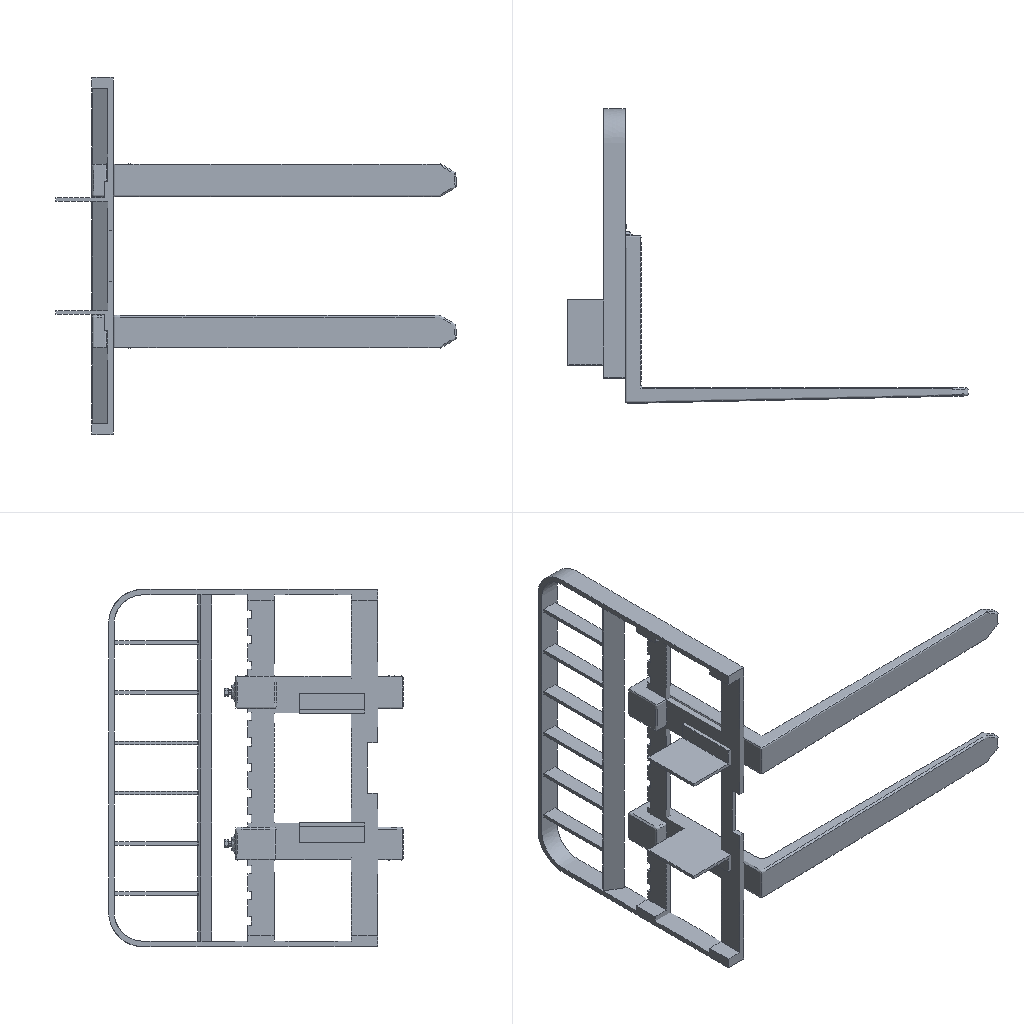Simulation study | ansys workbench
Set-up summary:
category,name,step,type,value,unit,region
solver,ansys_workbench
units,SI m-kg-s (Pa),,stated,"/units,MKS"
analysis,LS1,,static
load_step,LS1,LS1,static,nsubst=1; time=1
mesh,nodes,,,107409
mesh,elements,,,69133
element_type,SOLID187,,,59245
element_type,TARGE170,,,4743
element_type,CONTA174,,,4743
element_type,SOLID186,,,390
element_type,SURF154,,,12
material,Structural Steel,,E,2e+11,Pa
material,Structural Steel,,nu,0.3
material,Structural Steel,,density,7850,kg m^-3
material,Structural Steel,,conductivity,60.5,W m^-1 C^-1
material,Structural Steel,,specific_heat,434,J kg^-1 C^-1
material,Structural Steel,,cte,1.2e-05,C^-1
material,Structural Steel,,permeability,10000
material,Structural Steel,,resistivity,1.7e-07,kg m^3 A^-2 s^-3
load,Define Force Using Surface Effect Elements,LS1,surface-effect pres face 1,260906,,SURF154 #17
load,Define Force Using Surface Effect Elements,LS1,surface-effect pres face 2,-1.18334e+07,,SURF154 #17
bc,Fixed Supports,model,fixed,[dofs=ALL],,_FIXEDSU
contact,Contact Region 69,,bonded (always),element=CONTA174
contact,Contact Region 70,,bonded (always),element=CONTA174
contact,Contact Region 71,,bonded (always),element=CONTA174
contact,Contact Region 72,,bonded (always),element=CONTA174
contact,Contact Region 73,,bonded (always),element=CONTA174
named_set,_FIXEDSU,,node,1202
Ansys APDL input file, long lists of numbers shortened:
/batch
/config,noeldb,1     ! force off writing results to database
*get,_wallstrt,active,,time,wall
! ANSYS input file written by Workbench version 2024 R2
! File used for geometry attach:
/title,wbnew--____ (A5)
! ****** Begin Custom Load Command Snippet ******
/COM, ACT Extensions:
/COM,     LSDYNA, 2024.2
/COM,/COM,     ANSYSMotion, 2024.2
/COM,
! ****** End   Custom Load Command Snippet ******
*DIM,_wb_ProjectScratch_dir,string,248
_wb_ProjectScratch_dir(1) = ''
*DIM,_wb_SolverFiles_dir,string,248
_wb_SolverFiles_dir(1) = ''
*DIM,_wb_userfiles_dir,string,248
_wb_userfiles_dir(1) = ''
/com,--- Data in consistent MKS units. See Solving Units in the help system for more information.
/units,MKS
/nopr
/wb,file,start              !  signify a WB generated input file
/prep7
! Turn off shape checking because checks already performed inside WB mesher.
! See help system for more information.
SHPP,OFF,,NOWARN
/nolist
etcon,set             ! allow ANSYS to choose best KEYOP's for 180x elements, resets any applicable keyopt to MAPDL defaults
/com,*********** Nodes for the whole assembly ***********
nblock,3,,118149
(1i9,3e20.9e3)
   104394     6.272957041E-01     1.699172414E-01    -2.293882759E-01
! (107408 more lines like these left out)
-1
/wb,elem,start            !  set before creation of elements
/com,*********** Elements for Body 1 'EMPILHADEIRA_5T_ALTERADA_ASM_1_ASM|_______FORKLIFT_ASM_1_ASM|S_X_F3LIDO142_1|S_X_F3LIDO142_1' ***********
et,1,187
eblock,19,solid,,12218
(19i9)
        1        1        1        1        0        0        0        0       10        0        1      677     3666     4225     3693     8683    23642     8685     8684
! (24435 more lines like these left out)
-1
/com,*********** Elements for Body 2 'EMPILHADEIRA_5T_ALTERADA_ASM_1_ASM|_______FORKLIFT_ASM_1_ASM|S_X_F3LIDO143_1|S_X_F3LIDO143_1' ***********
et,2,187
eblock,19,solid,,18825
(19i9)
        2        2        2        2        0        0        0        0       10        0    12219    28224    29068    28415    28445    53792    54603    53786    53789
! (37649 more lines like these left out)
-1
/com,*********** Elements for Body 3 'EMPILHADEIRA_5T_ALTERADA_ASM_1_ASM|_______FORKLIFT_ASM_1_ASM|S_X_F3LIDO144_1|S_X_F3LIDO144_1' ***********
et,3,187
eblock,19,solid,,17962
(19i9)
        3        3        3        3        0        0        0        0       10        0    31044    58834    59006    59826    59181    82217    83239    82226    82221
! (35923 more lines like these left out)
-1
/com,*********** Elements for Body 4 'EMPILHADEIRA_5T_ALTERADA_ASM_1_ASM|_______FORKLIFT_ASM_1_ASM|S_X_F3LIDO152_1|S_X_F3LIDO152_1' ***********
et,4,187
eblock,19,solid,,10240
(19i9)
        4        4        4        4        0        0        0        0       10        0    49006    85338    88197    87604    88134    90879   103683    90876    90878
! (20479 more lines like these left out)
-1
/com,*********** Elements for Body 5 'EMPILHADEIRA_5T_ALTERADA_ASM_1_ASM|_______FORKLIFT_ASM_1_ASM|S_X_F3LIDO153_1|S_X_F3LIDO153_1' ***********
et,5,186
keyo,5,2,1          ! set full integration on SOLID186
eblock,19,solid,,195
(19i9)
        5        5        5        5        0        0        0        0       20        0    59246   104749   104790   104788   104775   104763   104838   104789   104776
! (389 more lines like these left out)
-1
/com,*********** Elements for Body 6 'EMPILHADEIRA_5T_ALTERADA_ASM_1_ASM|_______FORKLIFT_ASM_1_ASM|S_X_F3LIDO154_1|S_X_F3LIDO154_1' ***********
et,6,186
keyo,6,2,1          ! set full integration on SOLID186
eblock,19,solid,,195
(19i9)
        6        6        6        6        0        0        0        0       20        0    59441   106269   106311   106309   106296   106281   106349   106310   106297
! (389 more lines like these left out)
-1
/wb,elem,end               !  done creating elements
/com,*********** Send User Defined Coordinate System(s) ***********
csys,0
toffst,273.15,      ! Temperature offset from absolute zero
/com,*********** Set Reference Temperature ***********
tref,22.
/wb,mat,start              !  starting to send materials
/com,*********** Send Materials ***********
Temperature = 'TEMP' ! Temperature
MP,DENS,1,7850,	! kg m^-3
MP,ALPX,1,1.2e-05,	! C^-1
MP,C,1,434,	! J kg^-1 C^-1
MP,KXX,1,60.5,	! W m^-1 C^-1
MP,RSVX,1,1.7e-07,	! kg m^3 A^-2 s^-3
MP,EX,1,200000000000,	! Pa
MP,NUXY,1,0.3,
MP,MURX,1,10000,
Temperature = 'TEMP' ! Temperature
MP,DENS,2,7850,	! kg m^-3
MP,ALPX,2,1.2e-05,	! C^-1
MP,C,2,434,	! J kg^-1 C^-1
MP,KXX,2,60.5,	! W m^-1 C^-1
MP,RSVX,2,1.7e-07,	! kg m^3 A^-2 s^-3
MP,EX,2,200000000000,	! Pa
MP,NUXY,2,0.3,
MP,MURX,2,10000,
Temperature = 'TEMP' ! Temperature
MP,DENS,3,7850,	! kg m^-3
MP,ALPX,3,1.2e-05,	! C^-1
MP,C,3,434,	! J kg^-1 C^-1
MP,KXX,3,60.5,	! W m^-1 C^-1
MP,RSVX,3,1.7e-07,	! kg m^3 A^-2 s^-3
MP,EX,3,200000000000,	! Pa
MP,NUXY,3,0.3,
MP,MURX,3,10000,
Temperature = 'TEMP' ! Temperature
MP,DENS,4,7850,	! kg m^-3
MP,ALPX,4,1.2e-05,	! C^-1
MP,C,4,434,	! J kg^-1 C^-1
MP,KXX,4,60.5,	! W m^-1 C^-1
MP,RSVX,4,1.7e-07,	! kg m^3 A^-2 s^-3
MP,EX,4,200000000000,	! Pa
MP,NUXY,4,0.3,
MP,MURX,4,10000,
Temperature = 'TEMP' ! Temperature
MP,DENS,5,7850,	! kg m^-3
MP,ALPX,5,1.2e-05,	! C^-1
MP,C,5,434,	! J kg^-1 C^-1
MP,KXX,5,60.5,	! W m^-1 C^-1
MP,RSVX,5,1.7e-07,	! kg m^3 A^-2 s^-3
MP,EX,5,200000000000,	! Pa
MP,NUXY,5,0.3,
MP,MURX,5,10000,
Temperature = 'TEMP' ! Temperature
MP,DENS,6,7850,	! kg m^-3
MP,ALPX,6,1.2e-05,	! C^-1
MP,C,6,434,	! J kg^-1 C^-1
MP,KXX,6,60.5,	! W m^-1 C^-1
MP,RSVX,6,1.7e-07,	! kg m^3 A^-2 s^-3
MP,EX,6,200000000000,	! Pa
MP,NUXY,6,0.3,
MP,MURX,6,10000,
/wb,mat,end                !  done sending materials
!************************* Model Summary ********************
!EMPILHADEIRA_5T_ALTERADA_ASM_1_ASM|_______FORKLIFT_ASM_1_ASM|S_X_F3LIDO142_1|S_X_F3LIDO142_1,	ç»æé¢,	matid,	1
!EMPILHADEIRA_5T_ALTERADA_ASM_1_ASM|_______FORKLIFT_ASM_1_ASM|S_X_F3LIDO143_1|S_X_F3LIDO143_1,	ç»æé¢,	matid,	2
!EMPILHADEIRA_5T_ALTERADA_ASM_1_ASM|_______FORKLIFT_ASM_1_ASM|S_X_F3LIDO144_1|S_X_F3LIDO144_1,	ç»æé¢,	matid,	3
!EMPILHADEIRA_5T_ALTERADA_ASM_1_ASM|_______FORKLIFT_ASM_1_ASM|S_X_F3LIDO152_1|S_X_F3LIDO152_1,	ç»æé¢,	matid,	4
!EMPILHADEIRA_5T_ALTERADA_ASM_1_ASM|_______FORKLIFT_ASM_1_ASM|S_X_F3LIDO153_1|S_X_F3LIDO153_1,	ç»æé¢,	matid,	5
!EMPILHADEIRA_5T_ALTERADA_ASM_1_ASM|_______FORKLIFT_ASM_1_ASM|S_X_F3LIDO154_1|S_X_F3LIDO154_1,	ç»æé¢,	matid,	6
!************************* End Model Summary ********************
! get the diagonal of the bounding box. Needed later for other things
*get,_xmin,node,,mnloc,x
*get,_ymin,node,,mnloc,y
*get,_zmin,node,,mnloc,z
*get,_xmax,node,,mxloc,x
*get,_ymax,node,,mxloc,y
*get,_zmax,node,,mxloc,z
_ASMDIAG=(_xmax-_xmin)*(_xmax-_xmin)+(_ymax-_ymin)*(_ymax-_ymin)+(_zmax-_zmin)*(_zmax-_zmin)
_ASMDIAG=SQRT(_ASMDIAG)
/wb,contact,start          !  starting to send contact
/com,*********** Create Contact "½Ó´¥ÇøÓò 69" ***********
/com,            Real Constant Set For Above Contact Is 8 & 7
*set,tid,8
*set,cid,7
r,tid
r,cid
et,tid,170
et,cid,174
eblock,10,,,294
(15i9)
    84340        8        8        8        0      276     2404     2440     2440     6184    18024     2440     6185
! (293 more lines like these left out)
-1
eblock,10,,,294
(15i9)
    84634        7        7        7        0      276     2404     2440     2440     6184    18024     2440     6185
! (293 more lines like these left out)
-1
eblock,10,,,210
(15i9)
    84928        7        8        7        0    87600    87608    87609    87609   103650   103703    87609   103651
! (209 more lines like these left out)
-1
eblock,10,,,210
(15i9)
    85138        8        7        8        0    87600    87608    87609    87609   103650   103703    87609   103651
! (209 more lines like these left out)
-1
keyo,cid,8,2               ! auto create asymmetric contact (from Program Controlled setting)
keyo,cid,10,0              ! adjust contact stiffness each NR iteration (from Program Controlled setting)
keyo,cid,12,5              ! bonded always
keyo,cid,18,1              ! small sliding turned on by application
keyo,cid,2,2               ! MPC for bonded contacts (from Program Controlled setting)
keyo,tid,5,0               ! Automatic constraint type detection
keyo,cid,4,2               ! on nodal point - normal to target surface (from Program Controlled setting)
keyo,cid,9,1               ! ignore initial gaps/penetration
keyo,cid,7,0               ! No Prediction
rmod,tid,3,10.      ! FKN
rmod,tid,5,0.       ! ICONT
rmod,tid,6,0.       ! PINB
rmod,tid,10,0.      ! CNOF
rmod,tid,12,0.      ! FKT
rmod,tid,36,545     ! WB DSID
rmod,cid,3,10.      ! FKN
rmod,cid,5,0.       ! ICONT
rmod,cid,6,0.       ! PINB
rmod,cid,10,0.      ! CNOF
rmod,cid,12,0.      ! FKT
rmod,cid,36,545     ! WB DSID
/com,*********** Create Contact "½Ó´¥ÇøÓò 70" ***********
/com,            Real Constant Set For Above Contact Is 10 & 9
*set,tid,10
*set,cid,9
r,tid
r,cid
et,tid,170
et,cid,174
eblock,10,,,805
(15i9)
    85348       10       10       10        0    24960    24953    25250    25250    32885    32886    25250    32933
! (804 more lines like these left out)
-1
eblock,10,,,805
(15i9)
    86153        9        9        9        0    24960    24953    25250    25250    32885    32886    25250    32933
! (804 more lines like these left out)
-1
eblock,10,,,1010
(15i9)
    86958        9       10        9        0    86804    86976    87356    87356   100329   101434    87356   100331
! (1009 more lines like these left out)
-1
eblock,10,,,1010
(15i9)
    87968       10        9       10        0    86804    86976    87356    87356   100329   101434    87356   100331
! (1009 more lines like these left out)
-1
keyo,cid,8,2               ! auto create asymmetric contact (from Program Controlled setting)
keyo,cid,10,0              ! adjust contact stiffness each NR iteration (from Program Controlled setting)
keyo,cid,12,5              ! bonded always
keyo,cid,18,1              ! small sliding turned on by application
keyo,cid,2,2               ! MPC for bonded contacts (from Program Controlled setting)
keyo,tid,5,0               ! Automatic constraint type detection
keyo,cid,4,2               ! on nodal point - normal to target surface (from Program Controlled setting)
keyo,cid,9,1               ! ignore initial gaps/penetration
keyo,cid,7,0               ! No Prediction
rmod,tid,3,10.      ! FKN
rmod,tid,5,0.       ! ICONT
rmod,tid,6,0.       ! PINB
rmod,tid,10,0.      ! CNOF
rmod,tid,12,0.      ! FKT
rmod,tid,36,548     ! WB DSID
rmod,cid,3,10.      ! FKN
rmod,cid,5,0.       ! ICONT
rmod,cid,6,0.       ! PINB
rmod,cid,10,0.      ! CNOF
rmod,cid,12,0.      ! FKT
rmod,cid,36,548     ! WB DSID
/com,*********** Create Contact "½Ó´¥ÇøÓò 71" ***********
/com,            Real Constant Set For Above Contact Is 12 & 11
*set,tid,12
*set,cid,11
r,tid
r,cid
et,tid,170
et,cid,174
eblock,10,,,735
(15i9)
    88978       12       12       12        0    55916    55918    55920    55920    63635    63644    55920    63636
! (734 more lines like these left out)
-1
eblock,10,,,735
(15i9)
    89713       11       11       11        0    55916    55918    55920    55920    63635    63644    55920    63636
! (734 more lines like these left out)
-1
eblock,10,,,987
(15i9)
    90448       11       12       11        0    86766    87006    86856    86856   100071   100708    86856   100070
! (986 more lines like these left out)
-1
eblock,10,,,987
(15i9)
    91435       12       11       12        0    86766    87006    86856    86856   100071   100708    86856   100070
! (986 more lines like these left out)
-1
keyo,cid,8,2               ! auto create asymmetric contact (from Program Controlled setting)
keyo,cid,10,0              ! adjust contact stiffness each NR iteration (from Program Controlled setting)
keyo,cid,12,5              ! bonded always
keyo,cid,18,1              ! small sliding turned on by application
keyo,cid,2,2               ! MPC for bonded contacts (from Program Controlled setting)
keyo,tid,5,0               ! Automatic constraint type detection
keyo,cid,4,2               ! on nodal point - normal to target surface (from Program Controlled setting)
keyo,cid,9,1               ! ignore initial gaps/penetration
keyo,cid,7,0               ! No Prediction
rmod,tid,3,10.      ! FKN
rmod,tid,5,0.       ! ICONT
rmod,tid,6,0.       ! PINB
rmod,tid,10,0.      ! CNOF
rmod,tid,12,0.      ! FKT
rmod,tid,36,551     ! WB DSID
rmod,cid,3,10.      ! FKN
rmod,cid,5,0.       ! ICONT
rmod,cid,6,0.       ! PINB
rmod,cid,10,0.      ! CNOF
rmod,cid,12,0.      ! FKT
rmod,cid,36,551     ! WB DSID
/com,*********** Create Contact "½Ó´¥ÇøÓò 72" ***********
/com,            Real Constant Set For Above Contact Is 14 & 13
*set,tid,14
*set,cid,13
r,tid
r,cid
et,tid,170
et,cid,174
eblock,10,,,276
(15i9)
    92422       14       14       14        0    86715    87379    87163    87163    99683   102263    87163    99682
! (275 more lines like these left out)
-1
eblock,10,,,276
(15i9)
    92698       13       13       13        0    86715    87379    87163    87163    99683   102263    87163    99682
! (275 more lines like these left out)
-1
eblock,10,,,65
(15i9)
    92974       13       14       13        0   104838   104790   104788   104789   105817   105813   105812   105814
! (64 more lines like these left out)
-1
eblock,10,,,65
(15i9)
    93039       14       13       14        0   104838   104790   104788   104789   105817   105813   105812   105814
! (64 more lines like these left out)
-1
keyo,cid,8,2               ! auto create asymmetric contact (from Program Controlled setting)
keyo,cid,10,0              ! adjust contact stiffness each NR iteration (from Program Controlled setting)
keyo,cid,12,5              ! bonded always
keyo,cid,18,1              ! small sliding turned on by application
keyo,cid,2,2               ! MPC for bonded contacts (from Program Controlled setting)
keyo,tid,5,0               ! Automatic constraint type detection
keyo,cid,4,2               ! on nodal point - normal to target surface (from Program Controlled setting)
keyo,cid,9,1               ! ignore initial gaps/penetration
keyo,cid,7,0               ! No Prediction
rmod,tid,3,10.      ! FKN
rmod,tid,5,0.       ! ICONT
rmod,tid,6,0.       ! PINB
rmod,tid,10,0.      ! CNOF
rmod,tid,12,0.      ! FKT
rmod,tid,36,554     ! WB DSID
rmod,cid,3,10.      ! FKN
rmod,cid,5,0.       ! ICONT
rmod,cid,6,0.       ! PINB
rmod,cid,10,0.      ! CNOF
rmod,cid,12,0.      ! FKT
rmod,cid,36,554     ! WB DSID
/com,*********** Create Contact "½Ó´¥ÇøÓò 73" ***********
/com,            Real Constant Set For Above Contact Is 16 & 15
*set,tid,16
*set,cid,15
r,tid
r,cid
et,tid,170
et,cid,174
eblock,10,,,296
(15i9)
    93104       16       16       16        0    86804    86976    87356    87356   100329   101434    87356   100331
! (295 more lines like these left out)
-1
eblock,10,,,296
(15i9)
    93400       15       15       15        0    86804    86976    87356    87356   100329   101434    87356   100331
! (295 more lines like these left out)
-1
eblock,10,,,65
(15i9)
    93696       15       16       15        0   106284   106233   106231   106232   107161   107157   107156   107158
! (64 more lines like these left out)
-1
eblock,10,,,65
(15i9)
    93761       16       15       16        0   106284   106233   106231   106232   107161   107157   107156   107158
! (64 more lines like these left out)
-1
keyo,cid,8,2               ! auto create asymmetric contact (from Program Controlled setting)
keyo,cid,10,0              ! adjust contact stiffness each NR iteration (from Program Controlled setting)
keyo,cid,12,5              ! bonded always
keyo,cid,18,1              ! small sliding turned on by application
keyo,cid,2,2               ! MPC for bonded contacts (from Program Controlled setting)
keyo,tid,5,0               ! Automatic constraint type detection
keyo,cid,4,2               ! on nodal point - normal to target surface (from Program Controlled setting)
keyo,cid,9,1               ! ignore initial gaps/penetration
keyo,cid,7,0               ! No Prediction
rmod,tid,3,10.      ! FKN
rmod,tid,5,0.       ! ICONT
rmod,tid,6,0.       ! PINB
rmod,tid,10,0.      ! CNOF
rmod,tid,12,0.      ! FKT
rmod,tid,36,557     ! WB DSID
rmod,cid,3,10.      ! FKN
rmod,cid,5,0.       ! ICONT
rmod,cid,6,0.       ! PINB
rmod,cid,10,0.      ! CNOF
rmod,cid,12,0.      ! FKT
rmod,cid,36,557     ! WB DSID
nsel,all
esel,all
/wb,contact,end            !  done creating contacts
/golist
/wb,load,start             !  starting to send loads
/com,*********** Fixed Supports ***********
CMBLOCK,_FIXEDSU,NODE,     1202
(8i10)
    104399    104400    104401    104402    104403    104404    104405    104406
! (150 more lines like these left out)
cmsel,s,_FIXEDSU
d,all,all
nsel,all
/com,*********** Define Force Using Surface Effect Elements ***********
local,12,0,0.,0.,0.,0.,0.,0.
csys,0
et,17,154
mat,17
eblock,10,,,12
(15i9)
    93826       17       17       17       12    25080    25385    25383    25383    33745    35735    25383    33744
! (11 more lines like these left out)
-1
esel,s,type,,17
keyop,17,2,1        ! Apply load in local coordinate system
keyop,17,7,1        ! Use original area so load is constant in large deformation
esel,all
/gst,on,on
fini
*get,_numnode,node,0,count
*get,_numelem,elem,0,count
*get, _MAXELEMNUM, elem, 0, NUM, MAX
*get, _MAXNODENUM, node, 0, NUM, MAX
*get, _MAXELEMTYPE, etyp, 0, NUM, MAX
*get, _MAXREALCONST, rcon, 0, NUM, MAX
/go
/wb,load,end               !  done creating loads
/com,--- Number of total nodes = %_numnode%
/com,--- Number of contact elements = 9498
/com,--- Number of spring elements = 0
/com,--- Number of bearing elements = 0
/com,--- Number of solid elements = 59635
/com,--- Number of condensed parts = 0
/com,--- Number of total elements = %_numelem%
*get,_wallbsol,active,,time,wall
/com,****************************************************************************
/com,*************************    SOLUTION       ********************************
/com,****************************************************************************
/solu
antype,0                   ! static analysis
_thickRatio=0.333   ! Ratio of thick parts in the model
eqsl,sparse,,,,,1
cntr,print,1               ! print out contact info and also make no initial contact an error
dmpoption,emat,no             ! Don't combine emat file for DANSYS
dmpoption,esav,no             ! Don't combine esav file for DANSYS
nldiag,cont,iter           ! print out contact info each equilibrium iteration
rescontrol,,none                 ! Do not keep any restart files
/com,****************************************************
/com,******************* SOLVE FOR LS 1 OF 1 ****************
esel,s,type,,17
nsle
sfe,all,1,pres,1,260906.268
sfe,all,2,pres,1,-11833448.262
sfe,all,3,pres,1,0.
nsel,all
esel,all
/nopr
/gopr
nsub,1,1,1
time,1.
outres,erase
outres,all,none
outres,nsol,all,
outres,rsol,all
outres,eangl,all
outres,etmp,all
outres,veng,all
outres,strs,all,
outres,epel,all,
outres,eppl,all,
outres,cont,all,
! *********** WB SOLVE COMMAND ***********
! check interactive state
*get,ANSINTER_,active,,int
*if,ANSINTER_,ne,0,then
/eof
*endif
solve
/com *************** Write FE CONNECTORS *********
CEWRITE,file,ce,,INTE
/com,****************************************************
/com,*************** FINISHED SOLVE FOR LS 1 *************
*get,_wallasol,active,,time,wall
/nopr
*get,_numnode,node,0,count
*get,_numelem,elem,0,count
*get, _MAXELEMNUM, elem, 0, NUM, MAX
*get, _MAXNODENUM, node, 0, NUM, MAX,,,INTERNAL
*get, _MAXELEMTYPE, etyp, 0, NUM, MAX
*get, _MAXREALCONST, rcon, 0, NUM, MAX
*get,_NSOLTHREADS,active,0,ntfs
*get,_NSOLPROCESSES,active,0,npfs
/gopr
/post1
xmlo,ENCODING,ISO-8859-1
xmlo,parm
/xml,parm,xml
fini
/gopr
*get,_walldone,active,,time,wall
_preptime=(_wallbsol-_wallstrt)*3600
_solvtime=(_wallasol-_wallbsol)*3600
_posttime=(_walldone-_wallasol)*3600
_totaltim=(_walldone-_wallstrt)*3600
*get,_dlbratio,active,0,solu,dlbr
*get,_combtime,active,0,solu,comb
*get,_ssmode,active,0,solu,ssmm
*get,_ndofs,active,0,solu,ndof
*get,_sol_end_time,active,0,set,time
*if,_sol_end_time,eq,1.,then
/fclean				!clean distributed files
*endif
/com,--- Total number of nodes = %_numnode%
/com,--- Total number of elements = %_numelem%
/com,--- Element load balance ratio = %_dlbratio%
/com,--- Time to combine distributed files = %_combtime%
/com,--- Sparse memory mode = %_ssmode%
/com,--- Number of DOF = %_ndofs%
/wb,file,end               ! done with WB generated input
Results summary:
result,analyses[0].index,,,1
result,analyses[0].system,,,SYS
result,analyses[0].deck,,,deck.dat
result,analyses[0].solve_status,,,completed
result,analyses[0].analysis_type,,,static
result,analyses[0].physics,,,mechanical
result,analyses[0].unit_system,,,"MKS: m, kg, N, s, V, A, degC"
result,analyses[0].n_sets,,,1
result,analyses[0].load_steps[0].set,set=1,,1
result,analyses[0].load_steps[0].time_or_freq,set=1,,1
result,analyses[0].load_steps[0].max_displacement_magnitude,set=1,,0.02881
result,analyses[0].load_steps[0].max_von_mises_nodal,set=1,,3.63173e+08
result,analyses[0].load_steps[0].reaction_force_sum_xyz[1],set=1,,-440.857
result,analyses[0].load_steps[0].reaction_force_sum_xyz[2],set=1,,19995.1
result,analyses[0].load_steps[0].reaction_force_sum_xyz[3],set=1,,-1.67007e-05